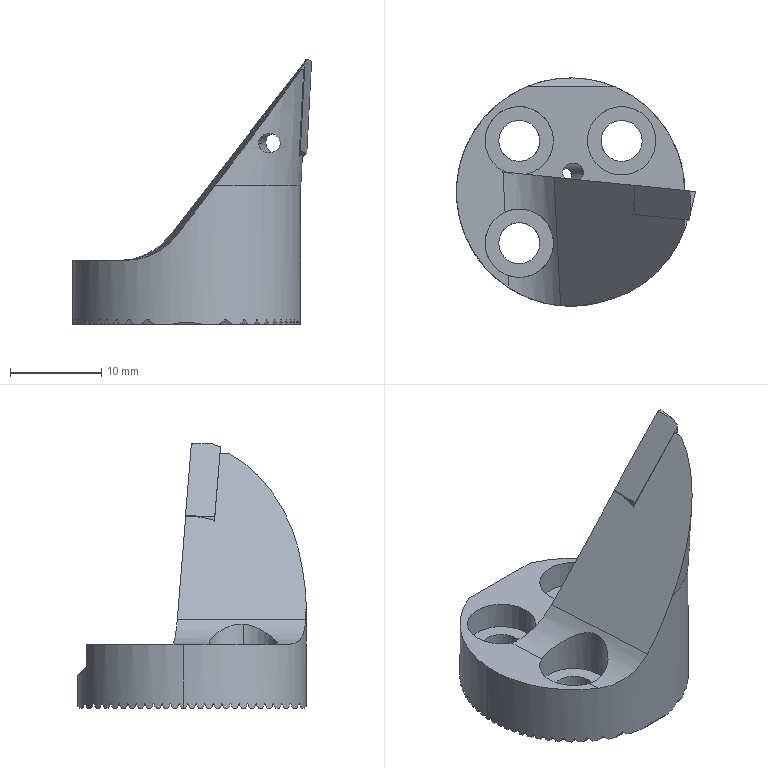NC program | Mastercam | posted with a generic post
Lines 1 to 736 of 4664:
%
:0001()
(MATERIAL - ALUMINUM MM - 2024)
(T4|12 FEMR |H4|XY STOCK TO LEAVE - 0.|Z STOCK TO LEAVE - .1)
(T1|6 FEM |H1|D1|WEAR COMP|TOOL DIA. - 6.)
(T2|2 DR |H2)
(T6|3 FEMR |H6|D6|WEAR COMP|TOOL DIA. - 3.|XY STOCK TO LEAVE - .1|Z STOCK TO LEAVE - .1)
(T7|3 FEMF |H7|D7|WEAR COMP|TOOL DIA. - 3.|XY STOCK TO LEAVE - 0.|Z STOCK TO LEAVE - .01)
(T8|2X7 DCHC |H8|D8|WEAR COMP|TOOL DIA. - 6.)
(T9|12 FEMF |H9|D9|WEAR COMP|TOOL DIA. - 12.)
(T10|30 BNOS |H10|D10|WEAR COMP|TOOL DIA. - 30.)
(T12|5 SPD |H12)
(T13|2.1 DR |H13)
(T11|2.5 FEM |H11)
(T14|1.95 THML |H14|D14|WEAR COMP|TOOL DIA. - 1.95)
(T15|2.5 BM |H15)
N100 G21
N102 G0 G17 G40 G80 G90 G94 G98
N104 G0 G28 G91 Z0.
N106 G0 G28 X0. Y0.
(12 FEMR |TOOL - 4|DIA. OFF. - 4|LEN. - 4|TOOL DIA. - 12.)
N108 T4 M6
N110 G0 G54 G90 X18.729 Y23.264 C6. B-90. S3500 M3
N112 G43 H4 Z61.514
N114 Z3.514
N116 G1 Z1.764 F2000.
N118 X18.032 Y21.694 Z1.613 F2500.
N120 G3 X17.8 Y20.599 Z1.514 I2.468 J-1.095
N122 G1 Y20.
N124 X18.056 Y19.941
N126 G3 X20.569 Y19.787 I2.632 J22.339
N128 X26.343 Y19.749 I5.774 J439.246
N130 X27.638 Y19.751 J439.284
N132 G1 X27.661
N134 G2 X30.947 Y18.812 J-6.222
N136 X33.523 Y16.129 I-3.997 J-6.415
N138 X34.711 Y12.875 I-9.239 J-5.217
N140 X35.088 Y9.299 I-22.374 J-4.17
N142 X35.163 Y3.723 I-206.196 J-5.576
N144 X35.161 Y2.708 I-206.271
N146 G1 X35.162 Y2.308
N148 X35.163 Y-12.263
N150 Y-12.266
N152 G2 X34.46 Y-15.114 I-6.124
N154 X31.871 Y-17.908 I-6.607 J3.527
N156 X28.543 Y-19.244 I-5.394 J8.625
N158 X25.119 Y-19.657 I-4.143 J19.95
N160 X19.998 Y-19.749 I-5.121 J143.095
N162 X19.283 Y-19.747 J143.187
N164 G1 X18.882
N166 X17.8 Y-19.749
N168 Y-20.547
N170 G3 X18.032 Y-21.642 Z1.588 I2.7
N172 G1 X18.729 Y-23.212 Z1.702
N174 G3 X19.206 Y-24.001 Z1.764 I3.34 J1.483
N176 X22.069 Y-25.384 I2.863 J2.272 F9500.
N178 X24.206 Y-24.694 J3.655
N180 G1 X34.599 Y-17.204
N182 G3 X36.767 Y-13.018 I-3.052 J4.236
N184 G1 X36.997 Y10.945
N186 G3 X36.998 Y11.053 I-11.3 J.108
N188 X28.764 Y21.929 I-11.301
N190 G1 X20.363 Y24.297
N192 G3 X20.027 Y24.343 I-.336 J-1.192
N194 X19.195 Y24.023 J-1.238
N196 X18.894 Y23.608 Z1.729 I.832 J-.918 F2500.
N198 G1 X18.729 Y23.235 Z1.702
N200 X18.032 Y21.666 Z1.588
N202 G3 X17.8 Y20.57 Z1.514 I2.468 J-1.096
N204 G1 Y19.971
N206 Y19.953
N208 G3 X18.517 Y19.777 I1.124 J3.02
N210 X21.399 Y19.558 I3.154 J22.437
N212 X25.999 Y19.504 I4.6 J196.075
N214 G1 X26.109
N216 G2 X31.955 Y16.835 I-.064 J-7.877
N218 X33.956 Y13.313 I-7.49 J-6.586
N220 X34.667 Y9.881 I-15.109 J-4.918
N222 X34.885 Y5.417 I-50.186 J-4.687
N224 X34.915 Y-2.243 I-967.073 J-7.66
N226 X34.913 Y-4.236 I-967.103
N228 G1 Y-4.635
N230 X34.912 Y-10.692
N232 G2 X32.241 Y-16.546 I-7.871 J.055
N234 X28.718 Y-18.545 I-6.583 J7.495
N236 X25.288 Y-19.254 I-4.914 J15.122
N238 X20.825 Y-19.472 I-4.686 J50.258
N240 G3 X18.663 Y-19.505 I.487 J-101.188
N242 X18.053 Y-19.563 I.837 J-12.046
N244 G1 X17.8 Y-19.586
N246 Y-20.384
N248 G3 X18.032 Y-21.479 Z1.588 I2.7
N250 G1 X18.729 Y-23.049 Z1.702
N252 G3 X19.207 Y-23.837 Z1.764 I3.3 J1.465
N254 X22.029 Y-25.195 I2.822 J2.253 F9500.
N256 X24.19 Y-24.477 J3.611
N258 G1 X34.317 Y-16.913
N260 G3 X36.387 Y-12.91 I-3.087 J4.133
N262 G1 X36.918 Y8.234
N264 G3 X36.923 Y8.596 I-14.406 J.362
N266 X27.244 Y22.208 I-14.411
N268 G1 X21.229 Y24.299
N270 G3 X20.573 Y24.41 I-.656 J-1.887
N272 X19.266 Y23.923 J-1.998
N274 X18.748 Y23.223 Z1.705 I1.307 J-1.511 F2500.
N276 G1 X18.729 Y23.18 Z1.702
N278 X18.032 Y21.611 Z1.588
N280 G3 X17.8 Y20.515 Z1.514 I2.468 J-1.096
N282 G1 Y19.917
N284 Y19.893
N286 G3 X18.493 Y19.673 I1.241 J2.713
N288 X21.187 Y19.364 I3.251 J16.412
N290 X24.589 Y19.272 I3.932 J82.803
N292 G1 X24.614
N294 G2 X27.653 Y18.811 J-10.244
N296 X32.259 Y15.301 I-2.839 J-8.502
N298 X33.861 Y11.732 I-9.779 J-6.535
N300 X34.464 Y8.064 I-19.652 J-5.114
N302 X34.644 Y2.898 I-74.541 J-5.185
N304 X34.663 Y-2.934 I-913.47 J-5.832
N306 X34.662 Y-3.932 I-913.489
N308 G1 Y-4.331
N310 G2 X34.664 Y-5.605 I-505.809 J-1.274
N312 X34.647 Y-9.759 I-505.811
N314 X30.992 Y-16.643 I-8.801 J.26
N316 X27.09 Y-18.462 I-6.781 J9.455
N318 X23.43 Y-19.055 I-5.094 J19.849
N320 X19.674 Y-19.228 I-5.416 J76.472
N322 G3 X17.8 Y-19.434 I.266 J-11.082
N324 G1 Y-19.833
N326 Y-20.232
N328 G3 X18.032 Y-21.327 Z1.588 I2.7
N330 G1 X18.729 Y-22.897 Z1.702
N332 G3 X19.202 Y-23.688 Z1.764 I3.476 J1.544
N334 X22.205 Y-25.157 I3.003 J2.335 F9500.
N336 X24.794 Y-24.14 J3.804
N338 G1 X34.461 Y-15.161
N340 G3 X36.196 Y-11.269 I-3.698 J3.981
N342 G1 X36.503 Y7.444
N344 G3 X36.505 Y7.694 I-15.24 J.25
N346 X27.347 Y21.669 I-15.242
N348 G1 X21.341 Y24.284
N350 G3 X20.572 Y24.444 I-.769 J-1.768
N352 X19.22 Y23.89 J-1.928
N354 X18.81 Y23.298 Z1.716 I1.352 J-1.374 F2500.
N356 G1 X18.729 Y23.115 Z1.702
N358 X18.032 Y21.545 Z1.588
N360 G3 X17.8 Y20.45 Z1.514 I2.468 J-1.095
N362 G1 Y19.851
N364 Y19.824
N366 G3 X18.473 Y19.57 I1.338 J2.534
N368 X21.027 Y19.181 I3.354 J13.446
N370 X23.613 Y19.056 I3.892 J53.394
N372 G2 X26.632 Y18.618 I-.235 J-12.263
N374 X31.952 Y14.648 I-2.695 J-9.16
N376 X33.578 Y10.931 I-10.521 J-6.818
N378 X34.22 Y6.853 I-22.103 J-5.568
N380 X34.395 Y1.402 I-84.615 J-5.451
N382 G1 Y1.317
N384 G2 X34.412 Y-4.433 I-974.808 J-5.75
N386 G1 Y-5.109
N388 Y-5.508
N390 G2 X34.415 Y-6.33 I-108.52 J-.822
N392 X34.388 Y-8.766 I-108.523
N394 X33.276 Y-13.019 I-10.064 J.36
N396 X29.549 Y-16.848 I-8.585 J4.627
N398 X26.164 Y-18.209 I-6.501 J11.279
N400 X22.127 Y-18.817 I-5.519 J22.931
N402 X20.114 Y-18.95 I-10.256 J140.669
N404 G3 X18.42 Y-19.144 I.944 J-15.69
N406 G2 X17.8 Y-19.285 I-8.324 J35.39
N408 G1 Y-19.684
N410 Y-20.083
N412 G3 X18.032 Y-21.178 Z1.588 I2.7
N414 G1 X18.729 Y-22.748 Z1.702
N416 G3 X19.199 Y-23.541 Z1.764 I3.611 J1.604
N418 X22.34 Y-25.095 I3.141 J2.397 F9500.
N420 X25.248 Y-23.82 J3.951
N422 G1 X34.456 Y-13.816
N424 G3 X35.948 Y-10.059 I-4.153 J3.823
N426 G1 X36.14 Y6.353
N428 G3 X36.141 Y6.553 I-17.036 J.2
N430 X26.305 Y21.993 I-17.037
N432 G1 X21.447 Y24.259
N434 G3 X20.621 Y24.442 I-.826 J-1.771
N436 X19.201 Y23.831 J-1.954
N438 X18.834 Y23.281 Z1.72 I1.42 J-1.343 F2500.
N440 G1 X18.729 Y23.043 Z1.702
N442 X18.032 Y21.474 Z1.588
N444 G3 X17.8 Y20.378 Z1.514 I2.468 J-1.096
N446 G1 Y19.779
N448 Y19.749
N450 G3 X18.454 Y19.468 I1.412 J2.381
N452 X20.897 Y19.009 I3.441 J11.575
N454 X23.141 Y18.839 I5.737 J61.024
N456 G2 X26.365 Y18.233 I-.72 J-12.707
N458 X31.632 Y14.092 I-3.275 J-9.586
N460 X33.23 Y10.475 I-11.014 J-7.025
N462 X33.925 Y6.399 I-21.838 J-5.824
N464 X34.138 Y.82 I-74.963 J-5.655
N466 X34.159 Y-4.114 I-569.499 J-4.934
N468 X34.15 Y-7.351 I-569.52
N470 X33.674 Y-10.672 I-12.746 J.135
N472 X29.631 Y-16.117 I-9.555 J2.87
N474 X25.992 Y-17.781 I-7.092 J10.698
N476 X22.41 Y-18.458 I-5.74 J20.556
N478 X20.021 Y-18.704 I-22.34 J205.155
N480 G3 X17.8 Y-19.136 I.974 J-10.933
N482 G1 Y-19.535
N484 Y-19.934
N486 G3 X18.032 Y-21.03 Z1.588 I2.7
N488 G1 X18.729 Y-22.599 Z1.702
N490 G3 X19.197 Y-23.395 Z1.764 I3.699 J1.642
N492 X22.428 Y-25.005 I3.231 J2.438 F9500.
N494 X25.551 Y-23.531 J4.048
N496 G1 X34.346 Y-12.857
N498 G3 X35.661 Y-9.42 I-4.461 J3.676
N500 G1 X36.375 Y7.779
N502 G3 X36.389 Y8.433 I-15.752 J.654
N504 X20.623 Y24.198 I-15.766
N506 X19.277 Y23.702 J-2.072
N508 X18.729 Y22.967 Z1.702 I1.346 J-1.576 F2500.
N510 G1 X18.032 Y21.397 Z1.588
N512 G3 X17.8 Y20.302 Z1.514 I2.468 J-1.095
N514 G1 Y19.703
N516 Y19.671
N518 G3 X18.435 Y19.366 I1.489 J2.285
N520 X20.788 Y18.843 I3.531 J10.323
N522 X23.189 Y18.574 I12.304 J99.065
N524 G2 X27.129 Y17.412 I-1.447 J-12.171
N526 X31.691 Y12.961 I-4.916 J-9.603
N528 X33.112 Y9.217 I-12.72 J-6.967
N530 X33.727 Y4.82 I-26.083 J-5.89
N532 X33.898 Y-1.289 I-108.917 J-6.109
N534 G1 Y-1.481
N536 G2 X33.908 Y-3.883 I-293.826 J-2.402
N538 X33.896 Y-6.436 I-293.836
N540 X33.446 Y-9.854 I-14.184 J.132
N542 X28.871 Y-15.957 I-10.039 J2.759
N544 X25.064 Y-17.582 I-7.222 J11.649
N546 X21.688 Y-18.221 I-6.602 J25.617
N548 G3 X18.935 Y-18.654 I3.936 J-34.006
N550 X17.8 Y-18.987 I1.595 J-7.537
N552 G1 Y-19.386
N554 Y-19.786
N556 G3 X18.032 Y-20.881 Z1.588 I2.7
N558 G1 X18.729 Y-22.451 Z1.702
N560 G3 X19.201 Y-23.243 Z1.764 I3.531 J1.568
N562 X22.26 Y-24.747 I3.059 J2.36 F9500.
N564 X25.183 Y-23.41 J3.864
N566 G1 X33.84 Y-13.399
N568 G3 X35.173 Y-10.149 I-4.175 J3.61
N570 G1 X35.988 Y2.32
N572 G3 X36.032 Y3.665 I-20.579 J1.345
N574 X25.967 Y21.38 I-20.623
N576 G1 X21.419 Y24.091
N578 G3 X20.517 Y24.34 I-.902 J-1.512
N580 X19.161 Y23.701 J-1.761
N582 X18.909 Y23.293 Z1.732 I1.356 J-1.122 F2500.
N584 G1 X18.729 Y22.887 Z1.702
N586 X18.032 Y21.318 Z1.588
N588 G3 X17.8 Y20.222 Z1.514 I2.468 J-1.096
N590 G1 Y19.624
N592 Y19.59
N594 G3 X18.417 Y19.264 I1.499 J2.089
N596 X20.712 Y18.678 I3.655 J9.522
N598 X22.245 Y18.453 I10.362 J65.229
N600 G2 X25.409 Y17.684 I-1.971 J-15.019
N602 X31.375 Y12.498 I-3.895 J-10.505
N604 X32.852 Y8.554 I-13.236 J-7.206
N606 X33.461 Y4.195 I-27.122 J-6.01
N608 X33.645 Y-2.033 I-105.423 J-6.228
N610 G1 Y-2.113
N612 G2 X33.654 Y-3.575 I-122.41 J-1.462
N614 X33.631 Y-5.935 I-122.419
N616 X33.161 Y-9.284 I-14.239 J.288
N618 X28.534 Y-15.549 I-10.397 J2.839
N620 X24.555 Y-17.287 I-7.601 J11.977
N622 X20.937 Y-18.038 I-9.255 J35.496
N624 G3 X18.506 Y-18.573 I2.894 J-18.939
N626 X17.8 Y-18.837 I3.089 J-9.354
N628 G1 Y-19.236
N630 Y-19.635
N632 G3 X18.032 Y-20.73 Z1.588 I2.7
N634 G1 X18.729 Y-22.3 Z1.702
N636 G3 X19.195 Y-23.096 Z1.764 I3.78 J1.679
N638 X22.509 Y-24.757 I3.314 J2.475 F9500.
N640 X25.881 Y-23.017 J4.136
N642 G1 X33.991 Y-11.603
N644 G3 X35.068 Y-8.601 I-4.817 J3.422
N646 G1 X35.742 Y.838
N648 G3 X35.799 Y2.441 I-22.464 J1.603
N650 X25.395 Y21.424 I-22.521
N652 G1 X21.376 Y23.99
N654 G3 X20.469 Y24.255 I-.907 J-1.422
N656 X19.153 Y23.623 J-1.687
N658 X18.927 Y23.253 Z1.735 I1.316 J-1.055 F2500.
N660 G1 X18.729 Y22.805 Z1.702
N662 X18.032 Y21.236 Z1.588
N664 G3 X17.8 Y20.14 Z1.514 I2.468 J-1.096
N666 G1 Y19.542
N668 Y19.507
N670 G3 X18.399 Y19.162 I1.543 J1.991
N672 X20.349 Y18.572 I3.688 J8.663
N674 G2 X22.772 Y18.095 I-33.73 J-177.815
N676 X26.36 Y16.796 I-2.783 J-13.294
N678 X31.221 Y11.769 I-5.587 J-10.266
N680 X32.707 Y7.402 I-14.561 J-7.392
N682 X33.253 Y2.708 I-32.851 J-6.2
N684 X33.388 Y-2.984 I-120.259 J-5.692
N686 X33.364 Y-5.382 I-120.394
N688 X32.804 Y-9.005 I-14.656 J.41
N690 X27.96 Y-15.312 I-10.659 J3.172
N692 X24.115 Y-16.995 I-7.899 J12.816
N694 X20.651 Y-17.814 I-12.867 J46.687
N696 G3 X18.379 Y-18.434 I3.065 J-15.685
N698 X17.974 Y-18.611 I3.795 J-9.253
N700 G1 X17.8 Y-18.684
N702 Y-19.482
N704 G3 X18.032 Y-20.577 Z1.588 I2.7
N706 G1 X18.729 Y-22.147 Z1.702
N708 G3 X19.24 Y-22.912 Z1.764 I2.468 J1.096
N710 G1 X19.559 Y-23.198 F9500.
N712 X19.919 Y-23.43
N714 X20.311 Y-23.602
N716 X20.725 Y-23.71
N718 X21.152 Y-23.751
N720 X21.579 Y-23.724
N722 X21.997 Y-23.63
N724 X22.395 Y-23.471
N726 X22.762 Y-23.252
N728 X23.091 Y-22.977
N730 X23.371 Y-22.653
N732 X23.597 Y-22.289
N734 X23.763 Y-21.894
N736 X23.864 Y-21.478
N738 X23.896 Y-21.051
N740 G2 X23.89 Y-20.332 I40.046 J.719
N742 X23.898 Y-19.53 I40.052
N744 X25.518 Y-17.512 I2.186 J-.096
N746 G3 X29.959 Y-14.998 I-4.68 J13.446
N748 X34.051 Y-7.751 I-7.799 J9.183
N750 X34.319 Y-4.482 I-19.766 J3.269
N752 G1 Y-4.405
N754 G3 X34.323 Y-3.36 I-127.149 J1.045
N756 X34.152 Y3.236 I-127.153
N758 X33.481 Y8.212 I-30.246 J-1.548
N760 X31.662 Y12.888 I-15.818 J-3.462
N762 X25.091 Y18.397 I-10.936 J-6.371
N764 G2 X23.896 Y20.329 I.965 J1.932
N766 G1 Y21.626
N768 G3 X21.197 Y24.325 I-2.699
N770 X19.24 Y23.486 J-2.699
N772 X18.729 Y22.721 Z1.702 I1.957 J-1.86 F2500.
N774 G1 X18.032 Y21.152 Z1.588
N776 G3 X17.8 Y20.056 Z1.514 I2.468 J-1.096
N778 G1 Y19.457
N780 Y19.421
N782 G3 X18.381 Y19.06 I1.583 J1.905
N784 X20.326 Y18.405 I4.003 J8.664
N786 X21.847 Y18.048 I19.124 J78.029
N788 G2 X25.371 Y16.843 I-3.456 J-15.866
N790 X30.915 Y11.355 I-5.315 J-10.915
N792 X32.452 Y6.791 I-15.189 J-7.653
N794 X32.993 Y2.124 I-33.94 J-6.299
N796 X33.122 Y-2.688 I-89.424 J-4.812
N798 X33.098 Y-4.784 I-89.553
N800 X32.471 Y-8.659 I-14.904 J.421
N802 X27.736 Y-14.87 I-10.917 J3.412
N804 X23.744 Y-16.704 I-8.455 J13.149
N806 X20.417 Y-17.599 I-19.241 J64.904
N808 G3 X18.285 Y-18.293 I3.268 J-13.642
N810 G2 X17.8 Y-18.528 I-5.657 J11.08
N812 G1 Y-18.927
N814 Y-19.326
N816 G3 X18.032 Y-20.422 Z1.588 I2.7
N818 G1 X18.729 Y-21.991 Z1.702
N820 G3 X19.24 Y-22.757 Z1.764 I2.468 J1.095
N822 G1 X19.559 Y-23.043 F9500.
N824 X19.919 Y-23.275
N826 X20.311 Y-23.447
N828 X20.725 Y-23.555
N830 X21.152 Y-23.596
N832 X21.579 Y-23.569
N834 X21.997 Y-23.475
N836 X22.395 Y-23.316
N838 X22.762 Y-23.097
N840 X23.091 Y-22.822
N842 X23.371 Y-22.498
N844 X23.597 Y-22.134
N846 X23.763 Y-21.739
N848 X23.864 Y-21.323
N850 X23.896 Y-20.896
N852 G2 X23.888 Y-20.03 I47.924 J.866
N854 X23.898 Y-19.082 I47.932
N856 X25.27 Y-17.152 I2.158 J-.082
N858 G3 X29.701 Y-14.545 I-5.07 J13.686
N860 X33.774 Y-7.216 I-8.144 J9.322
N862 X34.054 Y-3.817 I-20.475 J3.399
N864 G1 Y-3.802
N866 G3 X34.058 Y-2.948 I-90.198 J.854
N868 X33.823 Y3.571 I-90.202
N870 X32.988 Y8.557 I-26.913 J-1.943
N872 X30.794 Y13.361 I-15.178 J-4.029
N874 X25.041 Y18.021 I-10.776 J-7.423
N876 G2 X23.896 Y19.927 I1.015 J1.906
N878 G1 Y21.539
N880 G3 X21.197 Y24.238 I-2.699
N882 X19.24 Y23.4 J-2.699
N884 X18.729 Y22.635 Z1.702 I1.957 J-1.861 F2500.
N886 G1 X18.032 Y21.065 Z1.588
N888 G3 X17.8 Y19.97 Z1.514 I2.468 J-1.095
N890 G1 Y19.371
N892 Y19.334
N894 G3 X18.365 Y18.958 I1.622 J1.827
N896 X20.32 Y18.229 I4.454 J8.957
N898 X21.436 Y17.918 I31.235 J109.949
N900 G2 X24.732 Y16.734 I-4.688 J-18.233
N902 X30.753 Y10.684 I-5.468 J-11.462
N904 X32.199 Y6.198 I-16.113 J-7.671
N906 X32.757 Y1.124 I-35.969 J-6.523
N908 X32.853 Y-2.425 I-65.801 J-3.549
N910 X32.83 Y-4.147 I-65.897
N912 X32.264 Y-7.92 I-15.695 J.427
N914 X27.292 Y-14.589 I-11.303 J3.238
N916 X23.669 Y-16.332 I-8.79 J13.637
N918 X20.393 Y-17.337 I-22.916 J68.802
N920 G3 X18.281 Y-18.114 I3.755 J-13.478
N922 G2 X17.8 Y-18.37 I-7.44 J13.377
N924 G1 Y-18.769
N926 Y-19.168
N928 G3 X18.032 Y-20.264 Z1.588 I2.7
N930 G1 X18.729 Y-21.833 Z1.702
N932 G3 X19.193 Y-22.631 Z1.764 I3.877 J1.721
N934 X22.606 Y-24.354 I3.413 J2.519 F9500.
N936 X26.282 Y-22.229 J4.242
N938 G1 X33.34 Y-9.976
N940 G3 X34.065 Y-7.96 I-5.251 J3.025
N942 G1 X35.362 Y-.281
N944 G3 X35.604 Y2.61 I-17.116 J2.891
N946 X21.447 Y19.67 I-17.358
N948 G2 X20.561 Y20.737 I.2 J1.067
N950 X20.586 Y20.963 I1.086
N952 G1 X20.781 Y21.88
N954 G3 X20.805 Y22.107 I-1.061 J.227
N956 X19.72 Y23.192 I-1.085
N958 X19.399 Y23.143 J-1.085
N960 X18.729 Y22.547 Z1.702 I.321 J-1.036 F2500.
N962 G1 X18.032 Y20.977 Z1.588
N964 G3 X17.8 Y19.882 Z1.514 I2.468 J-1.095
N966 G1 Y19.283
N968 Y19.244
N970 G3 X18.352 Y18.853 I1.668 J1.769
N972 X20.322 Y18.043 I5.057 J9.5
N974 X21.046 Y17.809 I33.917 J103.487
N976 G2 X23.856 Y16.762 I-7.383 J-24.117
N978 X30.446 Y10.326 I-5.381 J-12.101
N980 X31.945 Y5.637 I-16.725 J-7.933
N982 X32.498 Y.582 I-37.039 J-6.608
N984 X32.575 Y-2.07 I-45.424 J-2.652
N986 X32.536 Y-3.962 I-45.501
N988 X31.768 Y-8.118 I-15.059 J.636
N990 X27.166 Y-14.111 I-11.384 J3.978
N992 X23.4 Y-16.038 I-9.536 J13.994
N994 X20.231 Y-17.123 I-25.467 J69.188
N996 G3 X18.222 Y-17.962 I3.963 J-12.314
N998 G1 X17.8 Y-18.209
N1000 Y-19.008
N1002 G3 X18.032 Y-20.103 Z1.588 I2.7
N1004 G1 X18.729 Y-21.673 Z1.702
N1006 G3 X19.222 Y-22.451 Z1.764 I2.862 J1.271
N1008 X21.591 Y-23.534 I2.369 J2.049 F9500.
N1010 X24.182 Y-22.161 J3.132
N1012 G1 X32.903 Y-9.318
N1014 G3 X33.989 Y-6.203 I-5.288 J3.59
N1016 G1 X34.335 Y-1.555
N1018 G3 X34.408 Y.419 I-26.475 J1.974
N1020 X25.355 Y20.388 I-26.548
N1022 G1 X21.552 Y23.72
N1024 G3 X20.501 Y24.115 I-1.051 J-1.199
N1026 X19.11 Y23.299 J-1.594
N1028 X19.044 Y23.168 Z1.754 I1.391 J-.778 F2500.
N1030 G1 X18.729 Y22.457 Z1.702
N1032 X18.032 Y20.888 Z1.588
N1034 G3 X17.8 Y19.792 Z1.514 I2.468 J-1.096
N1036 G1 Y19.193
N1038 Y19.153
N1040 G3 X18.342 Y18.745 I1.722 J1.722
N1042 X20.001 Y17.972 I4.952 J8.468
N1044 X21.459 Y17.43 I29.193 J76.215
N1046 G2 X24.842 Y15.846 I-6.864 J-19.074
N1048 X30.382 Y9.467 I-7.111 J-11.77
N1050 X31.737 Y4.85 I-18.254 J-7.865
N1052 X32.282 Y-1.882 I-41.311 J-6.732
N1054 X32.251 Y-3.487 I-41.856
N1056 X31.504 Y-7.605 I-15.088 J.614
N1058 X26.829 Y-13.789 I-11.713 J3.994
N1060 X22.959 Y-15.829 I-10.405 J15.051
N1062 X20.264 Y-16.844 I-32.806 J83.045
N1064 G3 X18.241 Y-17.764 I4.518 J-12.613
N1066 G2 X17.8 Y-18.045 I-7.27 J10.944
N1068 G1 Y-18.444
N1070 Y-18.843
N1072 G3 X18.032 Y-19.939 Z1.588 I2.7
N1074 G1 X18.729 Y-21.508 Z1.702
N1076 G3 X19.24 Y-22.273 Z1.764 I2.468 J1.095
N1078 X21.197 Y-23.113 I1.957 J1.86 F9500.
N1080 X23.896 Y-20.413 J2.7
N1082 G2 X23.884 Y-19.12 I69.68 J1.293
N1084 X23.898 Y-17.744 I69.692
N1086 X25.273 Y-15.804 I2.197 J-.099
N1088 G3 X29.483 Y-12.721 I-6.701 J13.57
N1090 X32.924 Y-5.783 I-9.699 J9.131
N1092 X33.224 Y-2.107 I-22.367 J3.676
N1094 X33.216 Y-1.53 I-22.667
N1096 X32.652 Y5.012 I-42.642 J-.384
N1098 X31.179 Y9.956 I-20.385 J-3.38
N1100 X24.974 Y16.844 I-13.443 J-5.873
N1102 G2 X23.896 Y18.713 I1.082 J1.869
N1104 G1 Y21.27
N1106 G3 X21.197 Y23.969 I-2.699
N1108 X19.24 Y23.13 J-2.699
N1110 X18.729 Y22.365 Z1.702 I1.957 J-1.86 F2500.
N1112 G1 X18.032 Y20.796 Z1.588
N1114 G3 X17.8 Y19.7 Z1.514 I2.468 J-1.096
N1116 G1 Y19.102
N1118 Y19.06
N1120 G3 X18.335 Y18.632 I1.79 J1.69
N1122 X20.003 Y17.786 I5.579 J8.934
N1124 X21.456 Y17.178 I42.595 J99.814
N1126 G2 X24.995 Y15.315 I-7.341 J-18.236
N1128 X29.834 Y9.673 I-7.981 J-11.74
N1130 X31.35 Y5.046 I-17.331 J-8.24
N1132 X31.986 Y-1.672 I-35.177 J-6.718
N1134 X31.961 Y-2.99 I-35.813
N1136 X31.137 Y-7.396 I-15.206 J.566
N1138 X26.763 Y-13.284 I-11.905 J4.274
N1140 X23.197 Y-15.347 I-10.866 J14.668
N1142 X20.143 Y-16.623 I-35.976 J81.78
N1144 G3 X18.178 Y-17.617 I4.671 J-11.686
N1146 X17.8 Y-18.038 I.679 J-.989
N1148 G1 Y-18.437
N1150 G3 X18.032 Y-19.532 Z1.588 I2.7
N1152 G1 X18.729 Y-21.101 Z1.702
N1154 Y-21.102
N1156 G3 X19.24 Y-21.867 Z1.764 I2.468 J1.096
N1158 G1 X19.559 Y-22.153 F9500.
N1160 X19.919 Y-22.385
N1162 X20.311 Y-22.557
N1164 X20.725 Y-22.665
N1166 X21.152 Y-22.706
N1168 X21.579 Y-22.679
N1170 X21.997 Y-22.585
N1172 X22.395 Y-22.426
N1174 X22.762 Y-22.207
N1176 X23.091 Y-21.932
N1178 X23.371 Y-21.608
N1180 X23.597 Y-21.244
N1182 X23.763 Y-20.849
N1184 X23.864 Y-20.433
N1186 X23.896 Y-20.006
N1188 G2 X23.89 Y-18.694 I138.848 J1.312
N1190 X23.897 Y-17.34 I138.854
N1192 X25.094 Y-15.446 I2.165 J-.043
N1194 G3 X29.2 Y-12.337 I-7.18 J13.747
N1196 X32.644 Y-5.274 I-9.972 J9.235
N1198 X32.926 Y-1.737 I-22.069 J3.537
N1200 X32.912 Y-.942 I-22.351
N1202 X32.246 Y5.298 I-37.116 J-.805
N1204 X30.416 Y10.576 I-19.414 J-3.774
N1206 X24.774 Y16.568 I-13.467 J-7.029
N1208 G2 X23.896 Y18.306 I1.282 J1.738
N1210 G1 Y21.175
N1212 G3 X21.197 Y23.874 I-2.699
N1214 X19.24 Y23.036 J-2.699
N1216 X18.729 Y22.271 Z1.702 I1.957 J-1.861 F2500.
N1218 G1 X18.032 Y20.702 Z1.588
N1220 G3 X17.8 Y19.606 Z1.514 I2.468 J-1.096
N1222 G1 Y19.007
N1224 Y18.964
N1226 G3 X18.331 Y18.514 I1.863 J1.661
N1228 X20.002 Y17.594 I6.21 J9.306
N1230 G2 X22.734 Y16.283 I-29.214 J-64.368
N1232 X26.954 Y13.132 I-7.097 J-13.907
N1234 X30.091 Y8.082 I-11.231 J-10.475
N1236 X31.344 Y3.105 I-21.484 J-8.056
N1238 X31.678 Y-1.428 I-30.582 J-4.533
N1240 X31.653 Y-2.679 I-30.916
N1242 X30.799 Y-7.102 I-15.066 J.614
N1244 X26.51 Y-12.924 I-12.173 J4.478
N1246 X22.834 Y-15.134 I-11.878 J15.597
N1248 X19.911 Y-16.461 I-45.812 J96.985
N1250 G3 X18.374 Y-17.312 I4. J-9.044
N1252 X17.885 Y-17.779 I.911 J-1.442
N1254 X17.8 Y-17.936 I1.009 J-.65
N1256 G1 Y-18.335
N1258 G3 X18.032 Y-19.431 Z1.588 I2.7
N1260 G1 X18.729 Y-21. Z1.702
N1262 G3 X19.212 Y-21.785 Z1.764 I3.17 J1.407
N1264 X21.899 Y-23.061 I2.687 J2.192 F9500.
N1266 X24.995 Y-21.156 J3.468
N1268 G1 X32.504 Y-6.281
N1270 G3 X33.259 Y-3.338 I-6.319 J3.189
N1272 X33.279 Y-2.218 I-32.127 J1.12
N1274 X27.524 Y16.135 I-32.147
N1276 G1 X23.04 Y22.584
N1278 G3 X21. Y23.65 I-2.04 J-1.419
N1280 X19.251 Y22.93 J-2.485
N1282 X18.729 Y22.174 Z1.702 I1.749 J-1.765 F2500.
N1284 G1 X18.032 Y20.604 Z1.588
N1286 G3 X17.8 Y19.509 Z1.514 I2.468 J-1.095
N1288 G1 Y18.91
N1290 Y18.864
N1292 G3 X18.327 Y18.391 I1.93 J1.622
N1294 X19.996 Y17.398 I6.792 J9.512
N1296 G2 X22.677 Y15.986 I-31.983 J-63.987
N1298 X26.719 Y12.802 I-7.967 J-14.274
N1300 X29.965 Y7.324 I-11.838 J-10.715
N1302 X31.177 Y1.903 I-23.081 J-8.007
N1304 X31.363 Y-1.107 I-24.2 J-3.01
N1306 X31.276 Y-3.167 I-24.386
N1308 X29.793 Y-8.32 I-13.918 J1.217
N1310 X26.285 Y-12.553 I-11.954 J6.337
N1312 X22.707 Y-14.82 I-12.563 J15.87
N1314 X19.853 Y-16.225 I-57.923 J114.058
N1316 G3 X18.383 Y-17.127 I3.945 J-8.077
N1318 G2 X17.8 Y-17.6 I-6.868 J7.878
N1320 G1 Y-17.999
N1322 Y-18.398
N1324 G3 X18.032 Y-19.493 Z1.588 I2.7
N1326 G1 X18.729 Y-21.063 Z1.702
N1328 G3 X19.206 Y-21.852 Z1.764 I3.336 J1.481
N1330 X22.065 Y-23.233 I2.859 J2.27 F9500.
N1332 X25.408 Y-21.046 J3.651
N1334 G1 X32.343 Y-5.203
N1336 G3 X32.968 Y-2.216 I-6.823 J2.987
N1338 G1 Y-2.165
N1340 G3 X27.71 Y15.529 I-33.156 J-.226
N1342 G1 X22.763 Y23.23
N1344 G3 X21.016 Y24.184 I-1.747 J-1.122
N1346 X19.104 Y22.918 J-2.076
N1348 G1 X18.729 Y22.072 Z1.702 F2500.
N1350 X18.032 Y20.503 Z1.588
N1352 G3 X17.8 Y19.407 Z1.514 I2.468 J-1.096
N1354 G1 Y18.809
N1356 Y18.76
N1358 G3 X18.323 Y18.263 I2.207 J1.801
N1360 X19.983 Y17.199 I7.449 J9.785
N1362 X20.999 Y16.633 I65.267 J116.072
N1364 G2 X24.355 Y14.478 I-11.701 J-21.916
N1366 X29.457 Y7.601 I-9.858 J-12.644
N1368 X30.824 Y2.127 I-21.459 J-8.269
N1370 X31.035 Y-.913 I-21.823 J-3.04
N1372 X30.927 Y-3.085 I-22.034
N1374 X28.828 Y-9.092 I-13.556 J1.368
N1376 X25.193 Y-12.871 I-12.233 J8.129
N1378 X21.819 Y-14.919 I-15.235 J21.296
N1380 G3 X19.321 Y-16.273 I19.587 J-39.115
N1382 X17.8 Y-17.403 I5.52 J-9.023
N1384 G1 Y-17.802
N1386 Y-18.201
N1388 G3 X18.032 Y-19.296 Z1.588 I2.7
N1390 G1 X18.729 Y-20.865 Z1.702
N1392 Y-20.866
N1394 G3 X19.24 Y-21.631 Z1.764 I2.468 J1.096
N1396 G1 X19.559 Y-21.917 F9500.
N1398 X19.919 Y-22.149
N1400 X20.311 Y-22.321
N1402 X20.725 Y-22.429
N1404 X21.152 Y-22.47
N1406 X21.579 Y-22.443
N1408 X21.997 Y-22.349
N1410 X22.395 Y-22.19
N1412 X22.762 Y-21.971
N1414 X23.091 Y-21.696
N1416 X23.371 Y-21.372
N1418 X23.597 Y-21.008
N1420 X23.763 Y-20.613
N1422 X23.864 Y-20.197
N1424 X23.896 Y-19.77
N1426 G2 X23.887 Y-17.9 I200.098 J1.87
N1428 X23.897 Y-15.989 I200.107
N1430 X24.882 Y-14.216 I2.16 J-.041
N1432 G3 X28.83 Y-10.677 I-8.7 J13.674
N1434 X31.835 Y-3.31 I-11.273 J8.896
N1436 X31.965 Y-.91 I-22.127 J2.4
N1438 X31.799 Y1.803 I-22.257
N1440 X30.307 Y7.975 I-23.973 J-2.529
N1442 X24.593 Y15.475 I-15.922 J-6.202
N1444 G2 X23.896 Y17.064 I1.463 J1.589
N1446 G1 Y20.872
N1448 G3 X21.197 Y23.571 I-2.699
N1450 X19.24 Y22.732 J-2.699
N1452 X18.729 Y21.967 Z1.702 I1.957 J-1.86 F2500.
N1454 G1 X18.032 Y20.398 Z1.588
N1456 G3 X17.8 Y19.302 Z1.514 I2.468 J-1.096
N1458 G1 Y18.703
N1460 Y18.652
N1462 G3 X18.496 Y17.986 I2.889 J2.325
N1464 X20.275 Y16.807 I9.978 J13.129
N1466 G1 X20.608 Y16.607
N1468 G2 X23.783 Y14.505 I-15.613 J-27.028
N1470 X29.354 Y6.819 I-10.156 J-13.224
N1472 X30.69 Y-.883 I-21.529 J-7.702
N1474 X30.668 Y-1.892 I-22.865
N1476 X29.324 Y-7.312 I-14.3 J.671
N1478 X25.866 Y-11.808 I-12.66 J6.16
N1480 X22.471 Y-14.194 I-14.072 J16.412
N1482 G3 X19.787 Y-15.735 I86.278 J-153.412
N1484 X18.089 Y-16.946 I5.78 J-9.9
N1486 G1 X17.8 Y-17.211
N1488 Y-18.009
N1490 G3 X18.032 Y-19.105 Z1.588 I2.7
N1492 G1 X18.729 Y-20.674 Z1.702
N1494 G3 X19.217 Y-21.456 Z1.764 I3.007 J1.335
N1496 X21.736 Y-22.629 I2.519 J2.117 F9500.
N1498 X24.682 Y-20.805 J3.29
N1500 G1 X30.997 Y-8.116
N1502 G3 X32.922 Y.073 I-16.454 J8.189
N1504 X30.415 Y9.338 I-18.379
N1506 G1 X22.971 Y22.092
N1508 G3 X20.91 Y23.275 I-2.061 J-1.203
N1510 X19.256 Y22.61 J-2.386
N1512 X18.729 Y21.857 Z1.702 I1.654 J-1.721 F2500.
N1514 G1 X18.032 Y20.288 Z1.588
N1516 G3 X17.8 Y19.192 Z1.514 I2.468 J-1.096
N1518 G1 Y18.594
N1520 Y18.539
N1522 G3 X18.488 Y17.842 I3.059 J2.331
N1524 X20.567 Y16.384 I13.16 J16.55
N1526 G2 X23.641 Y14.209 I-17.545 J-28.073
N1528 X29.237 Y6.047 I-10.912 J-13.48
N1530 X30.345 Y-.755 I-20.331 J-6.802
N1532 X30.339 Y-1.233 I-21.439
N1534 X29.015 Y-6.956 I-14.366 J.308
N1536 X25.866 Y-11.249 I-12.852 J6.126